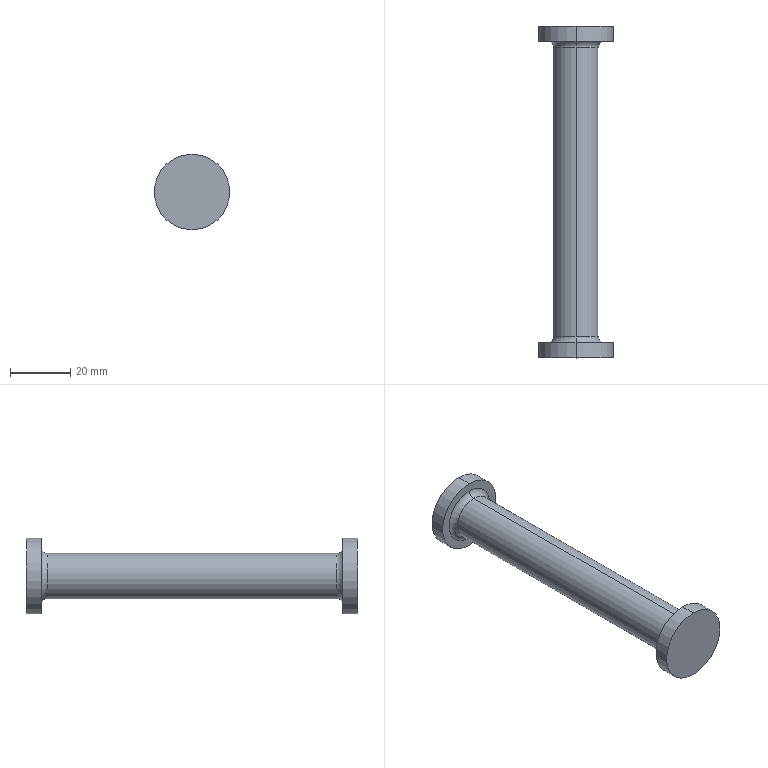Part | SolidWorks | features Fillet 1, Revolution 1 | 1 solid | 14 faces | box 25 x 110 x 25 mm | volume 22666 mm3 | cylinder 6 | torus 4 | plane 4 | commonest cylinder face diameters 25 x4 15 x2
STEP:
#1=CARTESIAN_POINT('',(0.,53.,7.5));
#2=VERTEX_POINT('',#1);
#3=CARTESIAN_POINT('',(0.,53.,-7.5));
#4=VERTEX_POINT('',#3);
#5=CARTESIAN_POINT('',(0.,53.,0.));
#6=DIRECTION('',(0.,-1.,0.));
#7=DIRECTION('',(0.,0.,-1.));
#8=AXIS2_PLACEMENT_3D('',#5,#6,#7);
#9=CIRCLE('',#8,7.5);
#10=EDGE_CURVE('',#2,#4,#9,.T.);
#11=ORIENTED_EDGE('',*,*,#10,.F.);
#12=CARTESIAN_POINT('',(0.,55.,9.5));
#13=VERTEX_POINT('',#12);
#14=CARTESIAN_POINT('',(0.,53.,9.5));
#15=DIRECTION('',(1.,0.,0.));
#16=DIRECTION('',(0.,0.,-1.));
#17=AXIS2_PLACEMENT_3D('',#14,#15,#16);
#18=CIRCLE('',#17,2.);
#19=EDGE_CURVE('',#2,#13,#18,.T.);
#20=ORIENTED_EDGE('',*,*,#19,.T.);
#21=CARTESIAN_POINT('',(0.,55.,-9.5));
#22=VERTEX_POINT('',#21);
#23=CARTESIAN_POINT('',(0.,55.,0.));
#24=DIRECTION('',(0.,1.,0.));
#25=DIRECTION('',(0.,0.,-1.));
#26=AXIS2_PLACEMENT_3D('',#23,#24,#25);
#27=CIRCLE('',#26,9.5);
#28=EDGE_CURVE('',#22,#13,#27,.T.);
#29=ORIENTED_EDGE('',*,*,#28,.F.);
#30=CARTESIAN_POINT('',(0.,53.,-9.5));
#31=DIRECTION('',(-1.,0.,0.));
#32=DIRECTION('',(0.,0.,1.));
#33=AXIS2_PLACEMENT_3D('',#30,#31,#32);
#34=CIRCLE('',#33,2.);
#35=EDGE_CURVE('',#4,#22,#34,.T.);
#36=ORIENTED_EDGE('',*,*,#35,.F.);
#37=EDGE_LOOP('',(#11,#20,#29,#36));
#38=FACE_OUTER_BOUND('',#37,.T.);
#39=CARTESIAN_POINT('',(0.,53.,0.));
#40=DIRECTION('',(0.,-1.,0.));
#41=DIRECTION('',(0.,0.,-1.));
#42=AXIS2_PLACEMENT_3D('',#39,#40,#41);
#43=TOROIDAL_SURFACE('',#42,9.5,2.);
#44=ADVANCED_FACE('',(#38),#43,.F.);
#45=CARTESIAN_POINT('',(0.,-43.,-7.5));
#46=VERTEX_POINT('',#45);
#47=CARTESIAN_POINT('',(0.,-43.,7.5));
#48=VERTEX_POINT('',#47);
#49=CARTESIAN_POINT('',(0.,-43.,0.));
#50=DIRECTION('',(0.,1.,0.));
#51=DIRECTION('',(0.,0.,1.));
#52=AXIS2_PLACEMENT_3D('',#49,#50,#51);
#53=CIRCLE('',#52,7.5);
#54=EDGE_CURVE('',#46,#48,#53,.T.);
#55=ORIENTED_EDGE('',*,*,#54,.F.);
#56=CARTESIAN_POINT('',(0.,-45.,-9.5));
#57=VERTEX_POINT('',#56);
#58=CARTESIAN_POINT('',(0.,-43.,-9.5));
#59=DIRECTION('',(1.,0.,0.));
#60=DIRECTION('',(0.,0.,-1.));
#61=AXIS2_PLACEMENT_3D('',#58,#59,#60);
#62=CIRCLE('',#61,2.);
#63=EDGE_CURVE('',#46,#57,#62,.T.);
#64=ORIENTED_EDGE('',*,*,#63,.T.);
#65=CARTESIAN_POINT('',(0.,-45.,9.5));
#66=VERTEX_POINT('',#65);
#67=CARTESIAN_POINT('',(0.,-45.,0.));
#68=DIRECTION('',(0.,-1.,0.));
#69=DIRECTION('',(0.,0.,1.));
#70=AXIS2_PLACEMENT_3D('',#67,#68,#69);
#71=CIRCLE('',#70,9.5);
#72=EDGE_CURVE('',#66,#57,#71,.T.);
#73=ORIENTED_EDGE('',*,*,#72,.F.);
#74=CARTESIAN_POINT('',(0.,-43.,9.5));
#75=DIRECTION('',(-1.,0.,0.));
#76=DIRECTION('',(0.,0.,1.));
#77=AXIS2_PLACEMENT_3D('',#74,#75,#76);
#78=CIRCLE('',#77,2.);
#79=EDGE_CURVE('',#48,#66,#78,.T.);
#80=ORIENTED_EDGE('',*,*,#79,.F.);
#81=EDGE_LOOP('',(#55,#64,#73,#80));
#82=FACE_OUTER_BOUND('',#81,.T.);
#83=CARTESIAN_POINT('',(0.,-43.,0.));
#84=DIRECTION('',(0.,1.,0.));
#85=DIRECTION('',(0.,0.,1.));
#86=AXIS2_PLACEMENT_3D('',#83,#84,#85);
#87=TOROIDAL_SURFACE('',#86,9.5,2.);
#88=ADVANCED_FACE('',(#82),#87,.F.);
#89=CARTESIAN_POINT('',(0.,-45.,-12.5));
#90=VERTEX_POINT('',#89);
#91=CARTESIAN_POINT('',(0.,-45.,12.5));
#92=VERTEX_POINT('',#91);
#93=CARTESIAN_POINT('',(0.,-45.,0.));
#94=DIRECTION('',(0.,-1.,0.));
#95=DIRECTION('',(0.,0.,-1.));
#96=AXIS2_PLACEMENT_3D('',#93,#94,#95);
#97=CIRCLE('',#96,12.5);
#98=EDGE_CURVE('',#90,#92,#97,.T.);
#99=ORIENTED_EDGE('',*,*,#98,.T.);
#100=CARTESIAN_POINT('',(0.,-50.,12.5));
#101=VERTEX_POINT('',#100);
#102=CARTESIAN_POINT('',(0.,-50.,12.5));
#103=DIRECTION('',(0.,-1.,0.));
#104=VECTOR('',#103,1000.);
#105=LINE('',#102,#104);
#106=EDGE_CURVE('',#92,#101,#105,.T.);
#107=ORIENTED_EDGE('',*,*,#106,.T.);
#108=CARTESIAN_POINT('',(0.,-50.,-12.5));
#109=VERTEX_POINT('',#108);
#110=CARTESIAN_POINT('',(0.,-50.,0.));
#111=DIRECTION('',(0.,-1.,0.));
#112=DIRECTION('',(0.,0.,-1.));
#113=AXIS2_PLACEMENT_3D('',#110,#111,#112);
#114=CIRCLE('',#113,12.5);
#115=EDGE_CURVE('',#109,#101,#114,.T.);
#116=ORIENTED_EDGE('',*,*,#115,.F.);
#117=CARTESIAN_POINT('',(0.,-50.,-12.5));
#118=DIRECTION('',(0.,-1.,0.));
#119=VECTOR('',#118,1000.);
#120=LINE('',#117,#119);
#121=EDGE_CURVE('',#90,#109,#120,.T.);
#122=ORIENTED_EDGE('',*,*,#121,.F.);
#123=EDGE_LOOP('',(#99,#107,#116,#122));
#124=FACE_OUTER_BOUND('',#123,.T.);
#125=CARTESIAN_POINT('',(0.,-50.,0.));
#126=DIRECTION('',(0.,-1.,0.));
#127=DIRECTION('',(0.,0.,-1.));
#128=AXIS2_PLACEMENT_3D('',#125,#126,#127);
#129=CYLINDRICAL_SURFACE('',#128,12.5);
#130=ADVANCED_FACE('',(#124),#129,.T.);
#131=CARTESIAN_POINT('',(0.,53.,0.));
#132=DIRECTION('',(0.,-1.,0.));
#133=DIRECTION('',(0.,0.,-1.));
#134=AXIS2_PLACEMENT_3D('',#131,#132,#133);
#135=CIRCLE('',#134,7.5);
#136=EDGE_CURVE('',#4,#2,#135,.T.);
#137=ORIENTED_EDGE('',*,*,#136,.T.);
#138=CARTESIAN_POINT('',(0.,-50.,7.5));
#139=DIRECTION('',(0.,-1.,0.));
#140=VECTOR('',#139,1000.);
#141=LINE('',#138,#140);
#142=EDGE_CURVE('',#2,#48,#141,.T.);
#143=ORIENTED_EDGE('',*,*,#142,.T.);
#144=CARTESIAN_POINT('',(0.,-43.,0.));
#145=DIRECTION('',(0.,1.,0.));
#146=DIRECTION('',(0.,0.,1.));
#147=AXIS2_PLACEMENT_3D('',#144,#145,#146);
#148=CIRCLE('',#147,7.5);
#149=EDGE_CURVE('',#48,#46,#148,.T.);
#150=ORIENTED_EDGE('',*,*,#149,.T.);
#151=CARTESIAN_POINT('',(0.,-50.,-7.5));
#152=DIRECTION('',(0.,-1.,0.));
#153=VECTOR('',#152,1000.);
#154=LINE('',#151,#153);
#155=EDGE_CURVE('',#4,#46,#154,.T.);
#156=ORIENTED_EDGE('',*,*,#155,.F.);
#157=EDGE_LOOP('',(#137,#143,#150,#156));
#158=FACE_OUTER_BOUND('',#157,.T.);
#159=CARTESIAN_POINT('',(0.,-50.,0.));
#160=DIRECTION('',(0.,-1.,0.));
#161=DIRECTION('',(0.,0.,-1.));
#162=AXIS2_PLACEMENT_3D('',#159,#160,#161);
#163=CYLINDRICAL_SURFACE('',#162,7.5);
#164=ADVANCED_FACE('',(#158),#163,.T.);
#165=CARTESIAN_POINT('',(0.,60.,-12.5));
#166=VERTEX_POINT('',#165);
#167=CARTESIAN_POINT('',(0.,60.,12.5));
#168=VERTEX_POINT('',#167);
#169=CARTESIAN_POINT('',(0.,60.,0.));
#170=DIRECTION('',(0.,-1.,0.));
#171=DIRECTION('',(0.,0.,-1.));
#172=AXIS2_PLACEMENT_3D('',#169,#170,#171);
#173=CIRCLE('',#172,12.5);
#174=EDGE_CURVE('',#166,#168,#173,.T.);
#175=ORIENTED_EDGE('',*,*,#174,.T.);
#176=CARTESIAN_POINT('',(0.,55.,12.5));
#177=VERTEX_POINT('',#176);
#178=CARTESIAN_POINT('',(0.,-50.,12.5));
#179=DIRECTION('',(0.,-1.,0.));
#180=VECTOR('',#179,1000.);
#181=LINE('',#178,#180);
#182=EDGE_CURVE('',#168,#177,#181,.T.);
#183=ORIENTED_EDGE('',*,*,#182,.T.);
#184=CARTESIAN_POINT('',(0.,55.,-12.5));
#185=VERTEX_POINT('',#184);
#186=CARTESIAN_POINT('',(0.,55.,0.));
#187=DIRECTION('',(0.,-1.,0.));
#188=DIRECTION('',(0.,0.,-1.));
#189=AXIS2_PLACEMENT_3D('',#186,#187,#188);
#190=CIRCLE('',#189,12.5);
#191=EDGE_CURVE('',#185,#177,#190,.T.);
#192=ORIENTED_EDGE('',*,*,#191,.F.);
#193=CARTESIAN_POINT('',(0.,-50.,-12.5));
#194=DIRECTION('',(0.,-1.,0.));
#195=VECTOR('',#194,1000.);
#196=LINE('',#193,#195);
#197=EDGE_CURVE('',#166,#185,#196,.T.);
#198=ORIENTED_EDGE('',*,*,#197,.F.);
#199=EDGE_LOOP('',(#175,#183,#192,#198));
#200=FACE_OUTER_BOUND('',#199,.T.);
#201=CARTESIAN_POINT('',(0.,-50.,0.));
#202=DIRECTION('',(0.,-1.,0.));
#203=DIRECTION('',(0.,0.,-1.));
#204=AXIS2_PLACEMENT_3D('',#201,#202,#203);
#205=CYLINDRICAL_SURFACE('',#204,12.5);
#206=ADVANCED_FACE('',(#200),#205,.T.);
#207=ORIENTED_EDGE('',*,*,#174,.F.);
#208=CARTESIAN_POINT('',(0.,60.,0.));
#209=DIRECTION('',(0.,-1.,0.));
#210=DIRECTION('',(0.,0.,-1.));
#211=AXIS2_PLACEMENT_3D('',#208,#209,#210);
#212=CIRCLE('',#211,12.5);
#213=EDGE_CURVE('',#168,#166,#212,.T.);
#214=ORIENTED_EDGE('',*,*,#213,.F.);
#215=EDGE_LOOP('',(#207,#214));
#216=FACE_OUTER_BOUND('',#215,.T.);
#217=CARTESIAN_POINT('',(0.,60.,0.));
#218=DIRECTION('',(0.,1.,0.));
#219=DIRECTION('',(0.,0.,1.));
#220=AXIS2_PLACEMENT_3D('',#217,#218,#219);
#221=PLANE('',#220);
#222=ADVANCED_FACE('',(#216),#221,.T.);
#223=ORIENTED_EDGE('',*,*,#182,.F.);
#224=ORIENTED_EDGE('',*,*,#213,.T.);
#225=ORIENTED_EDGE('',*,*,#197,.T.);
#226=CARTESIAN_POINT('',(0.,55.,0.));
#227=DIRECTION('',(0.,-1.,0.));
#228=DIRECTION('',(0.,0.,-1.));
#229=AXIS2_PLACEMENT_3D('',#226,#227,#228);
#230=CIRCLE('',#229,12.5);
#231=EDGE_CURVE('',#177,#185,#230,.T.);
#232=ORIENTED_EDGE('',*,*,#231,.F.);
#233=EDGE_LOOP('',(#223,#224,#225,#232));
#234=FACE_OUTER_BOUND('',#233,.T.);
#235=CARTESIAN_POINT('',(0.,-50.,0.));
#236=DIRECTION('',(0.,-1.,0.));
#237=DIRECTION('',(0.,0.,-1.));
#238=AXIS2_PLACEMENT_3D('',#235,#236,#237);
#239=CYLINDRICAL_SURFACE('',#238,12.5);
#240=ADVANCED_FACE('',(#234),#239,.T.);
#241=ORIENTED_EDGE('',*,*,#28,.T.);
#242=CARTESIAN_POINT('',(0.,55.,0.));
#243=DIRECTION('',(0.,1.,0.));
#244=DIRECTION('',(0.,0.,-1.));
#245=AXIS2_PLACEMENT_3D('',#242,#243,#244);
#246=CIRCLE('',#245,9.5);
#247=EDGE_CURVE('',#13,#22,#246,.T.);
#248=ORIENTED_EDGE('',*,*,#247,.T.);
#249=EDGE_LOOP('',(#241,#248));
#250=FACE_BOUND('',#249,.T.);
#251=ORIENTED_EDGE('',*,*,#191,.T.);
#252=ORIENTED_EDGE('',*,*,#231,.T.);
#253=EDGE_LOOP('',(#251,#252));
#254=FACE_OUTER_BOUND('',#253,.T.);
#255=CARTESIAN_POINT('',(12.5,55.,0.));
#256=DIRECTION('',(0.,-1.,0.));
#257=DIRECTION('',(0.,0.,-1.));
#258=AXIS2_PLACEMENT_3D('',#255,#256,#257);
#259=PLANE('',#258);
#260=ADVANCED_FACE('',(#250,#254),#259,.T.);
#261=ORIENTED_EDGE('',*,*,#142,.F.);
#262=ORIENTED_EDGE('',*,*,#10,.T.);
#263=ORIENTED_EDGE('',*,*,#155,.T.);
#264=ORIENTED_EDGE('',*,*,#54,.T.);
#265=EDGE_LOOP('',(#261,#262,#263,#264));
#266=FACE_OUTER_BOUND('',#265,.T.);
#267=CARTESIAN_POINT('',(0.,-50.,0.));
#268=DIRECTION('',(0.,-1.,0.));
#269=DIRECTION('',(0.,0.,-1.));
#270=AXIS2_PLACEMENT_3D('',#267,#268,#269);
#271=CYLINDRICAL_SURFACE('',#270,7.5);
#272=ADVANCED_FACE('',(#266),#271,.T.);
#273=ORIENTED_EDGE('',*,*,#72,.T.);
#274=CARTESIAN_POINT('',(0.,-45.,0.));
#275=DIRECTION('',(0.,-1.,0.));
#276=DIRECTION('',(0.,0.,1.));
#277=AXIS2_PLACEMENT_3D('',#274,#275,#276);
#278=CIRCLE('',#277,9.5);
#279=EDGE_CURVE('',#57,#66,#278,.T.);
#280=ORIENTED_EDGE('',*,*,#279,.T.);
#281=EDGE_LOOP('',(#273,#280));
#282=FACE_BOUND('',#281,.T.);
#283=ORIENTED_EDGE('',*,*,#98,.F.);
#284=CARTESIAN_POINT('',(0.,-45.,0.));
#285=DIRECTION('',(0.,-1.,0.));
#286=DIRECTION('',(0.,0.,-1.));
#287=AXIS2_PLACEMENT_3D('',#284,#285,#286);
#288=CIRCLE('',#287,12.5);
#289=EDGE_CURVE('',#92,#90,#288,.T.);
#290=ORIENTED_EDGE('',*,*,#289,.F.);
#291=EDGE_LOOP('',(#283,#290));
#292=FACE_OUTER_BOUND('',#291,.T.);
#293=CARTESIAN_POINT('',(12.5,-45.,0.));
#294=DIRECTION('',(0.,1.,0.));
#295=DIRECTION('',(0.,0.,1.));
#296=AXIS2_PLACEMENT_3D('',#293,#294,#295);
#297=PLANE('',#296);
#298=ADVANCED_FACE('',(#282,#292),#297,.T.);
#299=ORIENTED_EDGE('',*,*,#106,.F.);
#300=ORIENTED_EDGE('',*,*,#289,.T.);
#301=ORIENTED_EDGE('',*,*,#121,.T.);
#302=CARTESIAN_POINT('',(0.,-50.,0.));
#303=DIRECTION('',(0.,-1.,0.));
#304=DIRECTION('',(0.,0.,-1.));
#305=AXIS2_PLACEMENT_3D('',#302,#303,#304);
#306=CIRCLE('',#305,12.5);
#307=EDGE_CURVE('',#101,#109,#306,.T.);
#308=ORIENTED_EDGE('',*,*,#307,.F.);
#309=EDGE_LOOP('',(#299,#300,#301,#308));
#310=FACE_OUTER_BOUND('',#309,.T.);
#311=CARTESIAN_POINT('',(0.,-50.,0.));
#312=DIRECTION('',(0.,-1.,0.));
#313=DIRECTION('',(0.,0.,-1.));
#314=AXIS2_PLACEMENT_3D('',#311,#312,#313);
#315=CYLINDRICAL_SURFACE('',#314,12.5);
#316=ADVANCED_FACE('',(#310),#315,.T.);
#317=ORIENTED_EDGE('',*,*,#115,.T.);
#318=ORIENTED_EDGE('',*,*,#307,.T.);
#319=EDGE_LOOP('',(#317,#318));
#320=FACE_OUTER_BOUND('',#319,.T.);
#321=CARTESIAN_POINT('',(0.,-50.,0.));
#322=DIRECTION('',(0.,-1.,0.));
#323=DIRECTION('',(0.,0.,-1.));
#324=AXIS2_PLACEMENT_3D('',#321,#322,#323);
#325=PLANE('',#324);
#326=ADVANCED_FACE('',(#320),#325,.T.);
#327=ORIENTED_EDGE('',*,*,#63,.F.);
#328=ORIENTED_EDGE('',*,*,#149,.F.);
#329=ORIENTED_EDGE('',*,*,#79,.T.);
#330=ORIENTED_EDGE('',*,*,#279,.F.);
#331=EDGE_LOOP('',(#327,#328,#329,#330));
#332=FACE_OUTER_BOUND('',#331,.T.);
#333=CARTESIAN_POINT('',(0.,-43.,0.));
#334=DIRECTION('',(0.,1.,0.));
#335=DIRECTION('',(0.,0.,1.));
#336=AXIS2_PLACEMENT_3D('',#333,#334,#335);
#337=TOROIDAL_SURFACE('',#336,9.5,2.);
#338=ADVANCED_FACE('',(#332),#337,.F.);
#339=ORIENTED_EDGE('',*,*,#19,.F.);
#340=ORIENTED_EDGE('',*,*,#136,.F.);
#341=ORIENTED_EDGE('',*,*,#35,.T.);
#342=ORIENTED_EDGE('',*,*,#247,.F.);
#343=EDGE_LOOP('',(#339,#340,#341,#342));
#344=FACE_OUTER_BOUND('',#343,.T.);
#345=CARTESIAN_POINT('',(0.,53.,0.));
#346=DIRECTION('',(0.,-1.,0.));
#347=DIRECTION('',(0.,0.,-1.));
#348=AXIS2_PLACEMENT_3D('',#345,#346,#347);
#349=TOROIDAL_SURFACE('',#348,9.5,2.);
#350=ADVANCED_FACE('',(#344),#349,.F.);
#351=CLOSED_SHELL('',(#44,#88,#130,#164,#206,#222,#240,#260,#272,#298,#316,#326,#338,#350));
#352=MANIFOLD_SOLID_BREP('',#351);
#353=CARTESIAN_POINT('',(0.,0.,0.));
#354=DIRECTION('',(0.,0.,1.));
#355=DIRECTION('',(1.,0.,0.));
#356=AXIS2_PLACEMENT_3D('',#353,#354,#355);
#357=(LENGTH_UNIT()NAMED_UNIT(*)SI_UNIT(.MILLI.,.METRE.));
#358=UNCERTAINTY_MEASURE_WITH_UNIT(LENGTH_MEASURE(0.00001),#357,'','');
#359=(NAMED_UNIT(*)PLANE_ANGLE_UNIT()SI_UNIT($,.RADIAN.));
#360=(NAMED_UNIT(*)SI_UNIT($,.STERADIAN.)SOLID_ANGLE_UNIT());
#361=(GEOMETRIC_REPRESENTATION_CONTEXT(3)GLOBAL_UNCERTAINTY_ASSIGNED_CONTEXT((#358))GLOBAL_UNIT_ASSIGNED_CONTEXT((#357,#359,#360))REPRESENTATION_CONTEXT('',''));
#362=ADVANCED_BREP_SHAPE_REPRESENTATION('',(#352,#356),#361);